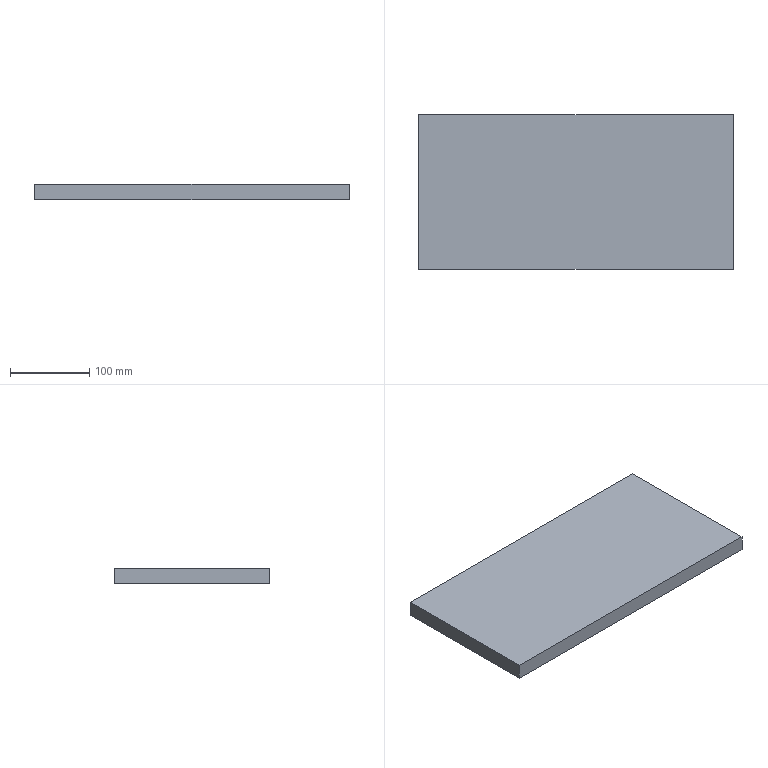Part | SolidWorks | features Extrusion 1 | 1 solid | 6 faces | box 398 x 195.319 x 20 mm | volume 1554736 mm3 | plane 6
STEP:
#1=CARTESIAN_POINT('',(-24.,42.,0.));
#2=VERTEX_POINT('',#1);
#3=CARTESIAN_POINT('',(-24.,-153.319,0.));
#4=VERTEX_POINT('',#3);
#5=CARTESIAN_POINT('',(-24.,42.,0.));
#6=DIRECTION('',(0.,-1.,0.));
#7=VECTOR('',#6,1000.);
#8=LINE('',#5,#7);
#9=EDGE_CURVE('',#2,#4,#8,.T.);
#10=ORIENTED_EDGE('',*,*,#9,.T.);
#11=CARTESIAN_POINT('',(-24.,-153.319,20.));
#12=VERTEX_POINT('',#11);
#13=CARTESIAN_POINT('',(-24.,-153.319,20.));
#14=DIRECTION('',(0.,0.,-1.));
#15=VECTOR('',#14,1000.);
#16=LINE('',#13,#15);
#17=EDGE_CURVE('',#12,#4,#16,.T.);
#18=ORIENTED_EDGE('',*,*,#17,.F.);
#19=CARTESIAN_POINT('',(-24.,42.,20.));
#20=VERTEX_POINT('',#19);
#21=CARTESIAN_POINT('',(-24.,42.,20.));
#22=DIRECTION('',(0.,-1.,0.));
#23=VECTOR('',#22,1000.);
#24=LINE('',#21,#23);
#25=EDGE_CURVE('',#20,#12,#24,.T.);
#26=ORIENTED_EDGE('',*,*,#25,.F.);
#27=CARTESIAN_POINT('',(-24.,42.,20.));
#28=DIRECTION('',(0.,0.,-1.));
#29=VECTOR('',#28,1000.);
#30=LINE('',#27,#29);
#31=EDGE_CURVE('',#20,#2,#30,.T.);
#32=ORIENTED_EDGE('',*,*,#31,.T.);
#33=EDGE_LOOP('',(#10,#18,#26,#32));
#34=FACE_OUTER_BOUND('',#33,.T.);
#35=CARTESIAN_POINT('',(-24.,42.,20.));
#36=DIRECTION('',(1.,0.,0.));
#37=DIRECTION('',(0.,0.,-1.));
#38=AXIS2_PLACEMENT_3D('',#35,#36,#37);
#39=PLANE('',#38);
#40=ADVANCED_FACE('',(#34),#39,.F.);
#41=CARTESIAN_POINT('',(374.,-153.319,0.));
#42=VERTEX_POINT('',#41);
#43=CARTESIAN_POINT('',(-24.,-153.319,0.));
#44=DIRECTION('',(1.,0.,0.));
#45=VECTOR('',#44,1000.);
#46=LINE('',#43,#45);
#47=EDGE_CURVE('',#4,#42,#46,.T.);
#48=ORIENTED_EDGE('',*,*,#47,.T.);
#49=CARTESIAN_POINT('',(374.,-153.319,20.));
#50=VERTEX_POINT('',#49);
#51=CARTESIAN_POINT('',(374.,-153.319,20.));
#52=DIRECTION('',(0.,0.,-1.));
#53=VECTOR('',#52,1000.);
#54=LINE('',#51,#53);
#55=EDGE_CURVE('',#50,#42,#54,.T.);
#56=ORIENTED_EDGE('',*,*,#55,.F.);
#57=CARTESIAN_POINT('',(-24.,-153.319,20.));
#58=DIRECTION('',(1.,0.,0.));
#59=VECTOR('',#58,1000.);
#60=LINE('',#57,#59);
#61=EDGE_CURVE('',#12,#50,#60,.T.);
#62=ORIENTED_EDGE('',*,*,#61,.F.);
#63=ORIENTED_EDGE('',*,*,#17,.T.);
#64=EDGE_LOOP('',(#48,#56,#62,#63));
#65=FACE_OUTER_BOUND('',#64,.T.);
#66=CARTESIAN_POINT('',(-24.,-153.319,20.));
#67=DIRECTION('',(0.,1.,0.));
#68=DIRECTION('',(0.,0.,1.));
#69=AXIS2_PLACEMENT_3D('',#66,#67,#68);
#70=PLANE('',#69);
#71=ADVANCED_FACE('',(#65),#70,.F.);
#72=CARTESIAN_POINT('',(374.,42.,0.));
#73=VERTEX_POINT('',#72);
#74=CARTESIAN_POINT('',(374.,42.,0.));
#75=DIRECTION('',(0.,1.,0.));
#76=VECTOR('',#75,1000.);
#77=LINE('',#74,#76);
#78=EDGE_CURVE('',#42,#73,#77,.T.);
#79=ORIENTED_EDGE('',*,*,#78,.T.);
#80=CARTESIAN_POINT('',(374.,42.,20.));
#81=VERTEX_POINT('',#80);
#82=CARTESIAN_POINT('',(374.,42.,20.));
#83=DIRECTION('',(0.,0.,-1.));
#84=VECTOR('',#83,1000.);
#85=LINE('',#82,#84);
#86=EDGE_CURVE('',#81,#73,#85,.T.);
#87=ORIENTED_EDGE('',*,*,#86,.F.);
#88=CARTESIAN_POINT('',(374.,42.,20.));
#89=DIRECTION('',(0.,1.,0.));
#90=VECTOR('',#89,1000.);
#91=LINE('',#88,#90);
#92=EDGE_CURVE('',#50,#81,#91,.T.);
#93=ORIENTED_EDGE('',*,*,#92,.F.);
#94=ORIENTED_EDGE('',*,*,#55,.T.);
#95=EDGE_LOOP('',(#79,#87,#93,#94));
#96=FACE_OUTER_BOUND('',#95,.T.);
#97=CARTESIAN_POINT('',(374.,42.,20.));
#98=DIRECTION('',(-1.,0.,0.));
#99=DIRECTION('',(0.,0.,1.));
#100=AXIS2_PLACEMENT_3D('',#97,#98,#99);
#101=PLANE('',#100);
#102=ADVANCED_FACE('',(#96),#101,.F.);
#103=CARTESIAN_POINT('',(-24.,42.,0.));
#104=DIRECTION('',(-1.,0.,0.));
#105=VECTOR('',#104,1000.);
#106=LINE('',#103,#105);
#107=EDGE_CURVE('',#73,#2,#106,.T.);
#108=ORIENTED_EDGE('',*,*,#107,.T.);
#109=ORIENTED_EDGE('',*,*,#31,.F.);
#110=CARTESIAN_POINT('',(-24.,42.,20.));
#111=DIRECTION('',(-1.,0.,0.));
#112=VECTOR('',#111,1000.);
#113=LINE('',#110,#112);
#114=EDGE_CURVE('',#81,#20,#113,.T.);
#115=ORIENTED_EDGE('',*,*,#114,.F.);
#116=ORIENTED_EDGE('',*,*,#86,.T.);
#117=EDGE_LOOP('',(#108,#109,#115,#116));
#118=FACE_OUTER_BOUND('',#117,.T.);
#119=CARTESIAN_POINT('',(-24.,42.,20.));
#120=DIRECTION('',(0.,-1.,0.));
#121=DIRECTION('',(0.,0.,-1.));
#122=AXIS2_PLACEMENT_3D('',#119,#120,#121);
#123=PLANE('',#122);
#124=ADVANCED_FACE('',(#118),#123,.F.);
#125=ORIENTED_EDGE('',*,*,#25,.T.);
#126=ORIENTED_EDGE('',*,*,#61,.T.);
#127=ORIENTED_EDGE('',*,*,#92,.T.);
#128=ORIENTED_EDGE('',*,*,#114,.T.);
#129=EDGE_LOOP('',(#125,#126,#127,#128));
#130=FACE_OUTER_BOUND('',#129,.T.);
#131=CARTESIAN_POINT('',(0.,0.,20.));
#132=DIRECTION('',(0.,0.,1.));
#133=DIRECTION('',(1.,0.,0.));
#134=AXIS2_PLACEMENT_3D('',#131,#132,#133);
#135=PLANE('',#134);
#136=ADVANCED_FACE('',(#130),#135,.T.);
#137=ORIENTED_EDGE('',*,*,#9,.F.);
#138=ORIENTED_EDGE('',*,*,#107,.F.);
#139=ORIENTED_EDGE('',*,*,#78,.F.);
#140=ORIENTED_EDGE('',*,*,#47,.F.);
#141=EDGE_LOOP('',(#137,#138,#139,#140));
#142=FACE_OUTER_BOUND('',#141,.T.);
#143=CARTESIAN_POINT('',(0.,0.,0.));
#144=DIRECTION('',(0.,0.,1.));
#145=DIRECTION('',(1.,0.,0.));
#146=AXIS2_PLACEMENT_3D('',#143,#144,#145);
#147=PLANE('',#146);
#148=ADVANCED_FACE('',(#142),#147,.F.);
#149=CLOSED_SHELL('',(#40,#71,#102,#124,#136,#148));
#150=MANIFOLD_SOLID_BREP('',#149);
#151=CARTESIAN_POINT('',(0.,0.,0.));
#152=DIRECTION('',(0.,0.,1.));
#153=DIRECTION('',(1.,0.,0.));
#154=AXIS2_PLACEMENT_3D('',#151,#152,#153);
#155=(LENGTH_UNIT()NAMED_UNIT(*)SI_UNIT(.MILLI.,.METRE.));
#156=UNCERTAINTY_MEASURE_WITH_UNIT(LENGTH_MEASURE(0.00001),#155,'','');
#157=(NAMED_UNIT(*)PLANE_ANGLE_UNIT()SI_UNIT($,.RADIAN.));
#158=(NAMED_UNIT(*)SI_UNIT($,.STERADIAN.)SOLID_ANGLE_UNIT());
#159=(GEOMETRIC_REPRESENTATION_CONTEXT(3)GLOBAL_UNCERTAINTY_ASSIGNED_CONTEXT((#156))GLOBAL_UNIT_ASSIGNED_CONTEXT((#155,#157,#158))REPRESENTATION_CONTEXT('',''));
#160=ADVANCED_BREP_SHAPE_REPRESENTATION('',(#150,#154),#159);